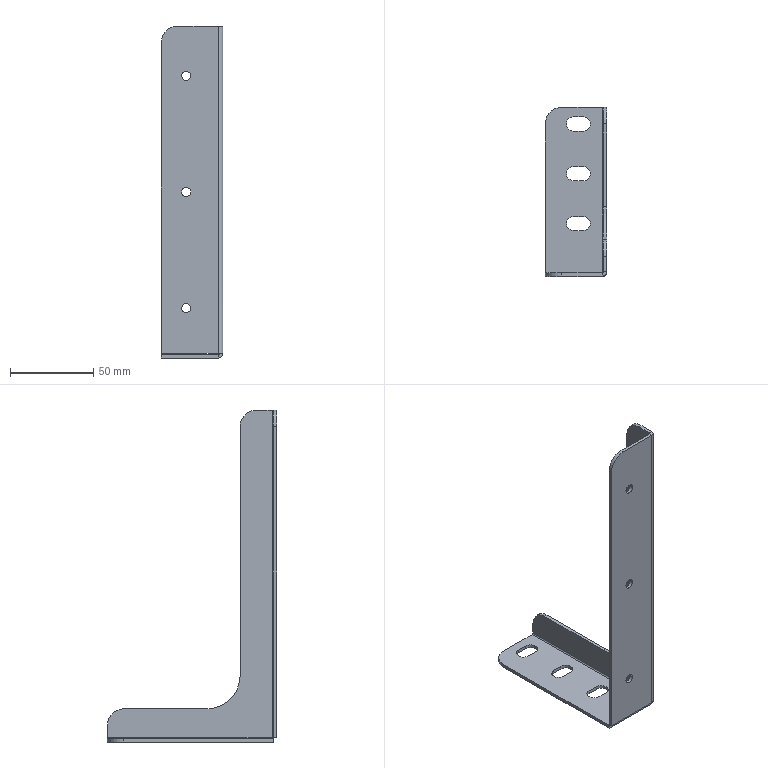Part | STEP file | 09-35 right support plate (Default) | 1 solid | 51 faces | box 37 x 102 x 200 mm | volume 31565 mm3 | plane 27 | cylinder 24 | commonest cylinder face diameters 8.5 x9 5.5 x6 20 x4 1.473 x2 5.473 x2 40 x1
STEP:
#1=CARTESIAN_POINT('',(9.75,-20.,-2.));
#2=VERTEX_POINT('',#1);
#3=CARTESIAN_POINT('',(5.5,-15.75,-2.));
#4=VERTEX_POINT('',#3);
#5=CARTESIAN_POINT('',(5.5,-20.,-2.));
#6=DIRECTION('',(0.,0.,1.));
#7=DIRECTION('',(1.,0.,0.));
#8=AXIS2_PLACEMENT_3D('',#5,#6,#7);
#9=CIRCLE('',#8,4.25);
#10=EDGE_CURVE('',#2,#4,#9,.T.);
#11=ORIENTED_EDGE('',*,*,#10,.F.);
#12=CARTESIAN_POINT('',(9.75,-20.,0.));
#13=VERTEX_POINT('',#12);
#14=CARTESIAN_POINT('',(9.75,-20.,-10.));
#15=DIRECTION('',(0.,0.,1.));
#16=VECTOR('',#15,1000.);
#17=LINE('',#14,#16);
#18=EDGE_CURVE('',#2,#13,#17,.T.);
#19=ORIENTED_EDGE('',*,*,#18,.T.);
#20=CARTESIAN_POINT('',(5.5,-15.75,0.));
#21=VERTEX_POINT('',#20);
#22=CARTESIAN_POINT('',(5.5,-20.,0.));
#23=DIRECTION('',(0.,0.,1.));
#24=DIRECTION('',(1.,0.,0.));
#25=AXIS2_PLACEMENT_3D('',#22,#23,#24);
#26=CIRCLE('',#25,4.25);
#27=EDGE_CURVE('',#13,#21,#26,.T.);
#28=ORIENTED_EDGE('',*,*,#27,.T.);
#29=CARTESIAN_POINT('',(5.5,-15.75,-10.));
#30=DIRECTION('',(0.,0.,1.));
#31=VECTOR('',#30,1000.);
#32=LINE('',#29,#31);
#33=EDGE_CURVE('',#4,#21,#32,.T.);
#34=ORIENTED_EDGE('',*,*,#33,.F.);
#35=EDGE_LOOP('',(#11,#19,#28,#34));
#36=FACE_OUTER_BOUND('',#35,.T.);
#37=CARTESIAN_POINT('',(5.5,-20.,-10.));
#38=DIRECTION('',(0.,0.,1.));
#39=DIRECTION('',(1.,0.,0.));
#40=AXIS2_PLACEMENT_3D('',#37,#38,#39);
#41=CYLINDRICAL_SURFACE('',#40,4.25);
#42=ADVANCED_FACE('',(#36),#41,.F.);
#43=CARTESIAN_POINT('',(9.75,10.,-2.));
#44=VERTEX_POINT('',#43);
#45=CARTESIAN_POINT('',(5.5,14.25,-2.));
#46=VERTEX_POINT('',#45);
#47=CARTESIAN_POINT('',(5.5,10.,-2.));
#48=DIRECTION('',(0.,0.,1.));
#49=DIRECTION('',(1.,0.,0.));
#50=AXIS2_PLACEMENT_3D('',#47,#48,#49);
#51=CIRCLE('',#50,4.25);
#52=EDGE_CURVE('',#44,#46,#51,.T.);
#53=ORIENTED_EDGE('',*,*,#52,.F.);
#54=CARTESIAN_POINT('',(9.75,10.,0.));
#55=VERTEX_POINT('',#54);
#56=CARTESIAN_POINT('',(9.75,10.,-10.));
#57=DIRECTION('',(0.,0.,1.));
#58=VECTOR('',#57,1000.);
#59=LINE('',#56,#58);
#60=EDGE_CURVE('',#44,#55,#59,.T.);
#61=ORIENTED_EDGE('',*,*,#60,.T.);
#62=CARTESIAN_POINT('',(5.5,14.25,0.));
#63=VERTEX_POINT('',#62);
#64=CARTESIAN_POINT('',(5.5,10.,0.));
#65=DIRECTION('',(0.,0.,1.));
#66=DIRECTION('',(1.,0.,0.));
#67=AXIS2_PLACEMENT_3D('',#64,#65,#66);
#68=CIRCLE('',#67,4.25);
#69=EDGE_CURVE('',#55,#63,#68,.T.);
#70=ORIENTED_EDGE('',*,*,#69,.T.);
#71=CARTESIAN_POINT('',(5.5,14.25,-10.));
#72=DIRECTION('',(0.,0.,1.));
#73=VECTOR('',#72,1000.);
#74=LINE('',#71,#73);
#75=EDGE_CURVE('',#46,#63,#74,.T.);
#76=ORIENTED_EDGE('',*,*,#75,.F.);
#77=EDGE_LOOP('',(#53,#61,#70,#76));
#78=FACE_OUTER_BOUND('',#77,.T.);
#79=CARTESIAN_POINT('',(5.5,10.,-10.));
#80=DIRECTION('',(0.,0.,1.));
#81=DIRECTION('',(1.,0.,0.));
#82=AXIS2_PLACEMENT_3D('',#79,#80,#81);
#83=CYLINDRICAL_SURFACE('',#82,4.25);
#84=ADVANCED_FACE('',(#78),#83,.F.);
#85=CARTESIAN_POINT('',(9.75,40.,-2.));
#86=VERTEX_POINT('',#85);
#87=CARTESIAN_POINT('',(5.5,44.25,-2.));
#88=VERTEX_POINT('',#87);
#89=CARTESIAN_POINT('',(5.5,40.,-2.));
#90=DIRECTION('',(0.,0.,1.));
#91=DIRECTION('',(1.,0.,0.));
#92=AXIS2_PLACEMENT_3D('',#89,#90,#91);
#93=CIRCLE('',#92,4.25);
#94=EDGE_CURVE('',#86,#88,#93,.T.);
#95=ORIENTED_EDGE('',*,*,#94,.F.);
#96=CARTESIAN_POINT('',(9.75,40.,0.));
#97=VERTEX_POINT('',#96);
#98=CARTESIAN_POINT('',(9.75,40.,-10.));
#99=DIRECTION('',(0.,0.,1.));
#100=VECTOR('',#99,1000.);
#101=LINE('',#98,#100);
#102=EDGE_CURVE('',#86,#97,#101,.T.);
#103=ORIENTED_EDGE('',*,*,#102,.T.);
#104=CARTESIAN_POINT('',(5.5,44.25,0.));
#105=VERTEX_POINT('',#104);
#106=CARTESIAN_POINT('',(5.5,40.,0.));
#107=DIRECTION('',(0.,0.,1.));
#108=DIRECTION('',(1.,0.,0.));
#109=AXIS2_PLACEMENT_3D('',#106,#107,#108);
#110=CIRCLE('',#109,4.25);
#111=EDGE_CURVE('',#97,#105,#110,.T.);
#112=ORIENTED_EDGE('',*,*,#111,.T.);
#113=CARTESIAN_POINT('',(5.5,44.25,-10.));
#114=DIRECTION('',(0.,0.,1.));
#115=VECTOR('',#114,1000.);
#116=LINE('',#113,#115);
#117=EDGE_CURVE('',#88,#105,#116,.T.);
#118=ORIENTED_EDGE('',*,*,#117,.F.);
#119=EDGE_LOOP('',(#95,#103,#112,#118));
#120=FACE_OUTER_BOUND('',#119,.T.);
#121=CARTESIAN_POINT('',(5.5,40.,-10.));
#122=DIRECTION('',(0.,0.,1.));
#123=DIRECTION('',(1.,0.,0.));
#124=AXIS2_PLACEMENT_3D('',#121,#122,#123);
#125=CYLINDRICAL_SURFACE('',#124,4.25);
#126=ADVANCED_FACE('',(#120),#125,.F.);
#127=CARTESIAN_POINT('',(-5.25,-50.,28.));
#128=VERTEX_POINT('',#127);
#129=CARTESIAN_POINT('',(0.25,-50.,28.));
#130=VERTEX_POINT('',#129);
#131=CARTESIAN_POINT('',(-2.5,-50.,28.));
#132=DIRECTION('',(0.,-1.,0.));
#133=DIRECTION('',(1.,0.,0.));
#134=AXIS2_PLACEMENT_3D('',#131,#132,#133);
#135=CIRCLE('',#134,2.75);
#136=EDGE_CURVE('',#128,#130,#135,.T.);
#137=ORIENTED_EDGE('',*,*,#136,.F.);
#138=CARTESIAN_POINT('',(-5.25,-52.,28.));
#139=VERTEX_POINT('',#138);
#140=CARTESIAN_POINT('',(-5.25,-42.,28.));
#141=DIRECTION('',(0.,-1.,0.));
#142=VECTOR('',#141,1000.);
#143=LINE('',#140,#142);
#144=EDGE_CURVE('',#128,#139,#143,.T.);
#145=ORIENTED_EDGE('',*,*,#144,.T.);
#146=CARTESIAN_POINT('',(0.25,-52.,28.));
#147=VERTEX_POINT('',#146);
#148=CARTESIAN_POINT('',(-2.5,-52.,28.));
#149=DIRECTION('',(0.,-1.,0.));
#150=DIRECTION('',(1.,0.,0.));
#151=AXIS2_PLACEMENT_3D('',#148,#149,#150);
#152=CIRCLE('',#151,2.75);
#153=EDGE_CURVE('',#139,#147,#152,.T.);
#154=ORIENTED_EDGE('',*,*,#153,.T.);
#155=CARTESIAN_POINT('',(0.25,-42.,28.));
#156=DIRECTION('',(0.,-1.,0.));
#157=VECTOR('',#156,1000.);
#158=LINE('',#155,#157);
#159=EDGE_CURVE('',#130,#147,#158,.T.);
#160=ORIENTED_EDGE('',*,*,#159,.F.);
#161=EDGE_LOOP('',(#137,#145,#154,#160));
#162=FACE_OUTER_BOUND('',#161,.T.);
#163=CARTESIAN_POINT('',(-2.5,-42.,28.));
#164=DIRECTION('',(0.,-1.,0.));
#165=DIRECTION('',(1.,0.,0.));
#166=AXIS2_PLACEMENT_3D('',#163,#164,#165);
#167=CYLINDRICAL_SURFACE('',#166,2.75);
#168=ADVANCED_FACE('',(#162),#167,.F.);
#169=CARTESIAN_POINT('',(-5.25,-50.,98.));
#170=VERTEX_POINT('',#169);
#171=CARTESIAN_POINT('',(0.25,-50.,98.));
#172=VERTEX_POINT('',#171);
#173=CARTESIAN_POINT('',(-2.5,-50.,98.));
#174=DIRECTION('',(0.,-1.,0.));
#175=DIRECTION('',(1.,0.,0.));
#176=AXIS2_PLACEMENT_3D('',#173,#174,#175);
#177=CIRCLE('',#176,2.75);
#178=EDGE_CURVE('',#170,#172,#177,.T.);
#179=ORIENTED_EDGE('',*,*,#178,.F.);
#180=CARTESIAN_POINT('',(-5.25,-52.,98.));
#181=VERTEX_POINT('',#180);
#182=CARTESIAN_POINT('',(-5.25,-42.,98.));
#183=DIRECTION('',(0.,-1.,0.));
#184=VECTOR('',#183,1000.);
#185=LINE('',#182,#184);
#186=EDGE_CURVE('',#170,#181,#185,.T.);
#187=ORIENTED_EDGE('',*,*,#186,.T.);
#188=CARTESIAN_POINT('',(0.25,-52.,98.));
#189=VERTEX_POINT('',#188);
#190=CARTESIAN_POINT('',(-2.5,-52.,98.));
#191=DIRECTION('',(0.,-1.,0.));
#192=DIRECTION('',(1.,0.,0.));
#193=AXIS2_PLACEMENT_3D('',#190,#191,#192);
#194=CIRCLE('',#193,2.75);
#195=EDGE_CURVE('',#181,#189,#194,.T.);
#196=ORIENTED_EDGE('',*,*,#195,.T.);
#197=CARTESIAN_POINT('',(0.25,-42.,98.));
#198=DIRECTION('',(0.,-1.,0.));
#199=VECTOR('',#198,1000.);
#200=LINE('',#197,#199);
#201=EDGE_CURVE('',#172,#189,#200,.T.);
#202=ORIENTED_EDGE('',*,*,#201,.F.);
#203=EDGE_LOOP('',(#179,#187,#196,#202));
#204=FACE_OUTER_BOUND('',#203,.T.);
#205=CARTESIAN_POINT('',(-2.5,-42.,98.));
#206=DIRECTION('',(0.,-1.,0.));
#207=DIRECTION('',(1.,0.,0.));
#208=AXIS2_PLACEMENT_3D('',#205,#206,#207);
#209=CYLINDRICAL_SURFACE('',#208,2.75);
#210=ADVANCED_FACE('',(#204),#209,.F.);
#211=CARTESIAN_POINT('',(-5.25,-50.,168.));
#212=VERTEX_POINT('',#211);
#213=CARTESIAN_POINT('',(0.25,-50.,168.));
#214=VERTEX_POINT('',#213);
#215=CARTESIAN_POINT('',(-2.5,-50.,168.));
#216=DIRECTION('',(0.,-1.,0.));
#217=DIRECTION('',(1.,0.,0.));
#218=AXIS2_PLACEMENT_3D('',#215,#216,#217);
#219=CIRCLE('',#218,2.75);
#220=EDGE_CURVE('',#212,#214,#219,.T.);
#221=ORIENTED_EDGE('',*,*,#220,.F.);
#222=CARTESIAN_POINT('',(-5.25,-52.,168.));
#223=VERTEX_POINT('',#222);
#224=CARTESIAN_POINT('',(-5.25,-42.,168.));
#225=DIRECTION('',(0.,-1.,0.));
#226=VECTOR('',#225,1000.);
#227=LINE('',#224,#226);
#228=EDGE_CURVE('',#212,#223,#227,.T.);
#229=ORIENTED_EDGE('',*,*,#228,.T.);
#230=CARTESIAN_POINT('',(0.25,-52.,168.));
#231=VERTEX_POINT('',#230);
#232=CARTESIAN_POINT('',(-2.5,-52.,168.));
#233=DIRECTION('',(0.,-1.,0.));
#234=DIRECTION('',(1.,0.,0.));
#235=AXIS2_PLACEMENT_3D('',#232,#233,#234);
#236=CIRCLE('',#235,2.75);
#237=EDGE_CURVE('',#223,#231,#236,.T.);
#238=ORIENTED_EDGE('',*,*,#237,.T.);
#239=CARTESIAN_POINT('',(0.25,-42.,168.));
#240=DIRECTION('',(0.,-1.,0.));
#241=VECTOR('',#240,1000.);
#242=LINE('',#239,#241);
#243=EDGE_CURVE('',#214,#231,#242,.T.);
#244=ORIENTED_EDGE('',*,*,#243,.F.);
#245=EDGE_LOOP('',(#221,#229,#238,#244));
#246=FACE_OUTER_BOUND('',#245,.T.);
#247=CARTESIAN_POINT('',(-2.5,-42.,168.));
#248=DIRECTION('',(0.,-1.,0.));
#249=DIRECTION('',(1.,0.,0.));
#250=AXIS2_PLACEMENT_3D('',#247,#248,#249);
#251=CYLINDRICAL_SURFACE('',#250,2.75);
#252=ADVANCED_FACE('',(#246),#251,.F.);
#253=CARTESIAN_POINT('',(19.5,-50.,0.7366));
#254=VERTEX_POINT('',#253);
#255=CARTESIAN_POINT('',(19.5,-49.263,0.7366));
#256=VERTEX_POINT('',#255);
#257=CARTESIAN_POINT('',(19.5,50.,0.7366));
#258=DIRECTION('',(0.,1.,0.));
#259=VECTOR('',#258,1000.);
#260=LINE('',#257,#259);
#261=EDGE_CURVE('',#254,#256,#260,.T.);
#262=ORIENTED_EDGE('',*,*,#261,.T.);
#263=CARTESIAN_POINT('',(19.399,-50.,0.7366));
#264=VERTEX_POINT('',#263);
#265=CARTESIAN_POINT('',(16.763,-49.263,0.7366));
#266=DIRECTION('',(0.,0.,-1.));
#267=DIRECTION('',(1.,0.,0.));
#268=AXIS2_PLACEMENT_3D('',#265,#266,#267);
#269=CIRCLE('',#268,2.737);
#270=EDGE_CURVE('',#256,#264,#269,.T.);
#271=ORIENTED_EDGE('',*,*,#270,.T.);
#272=CARTESIAN_POINT('',(17.5,-50.,0.7366));
#273=DIRECTION('',(1.,0.,0.));
#274=VECTOR('',#273,1000.);
#275=LINE('',#272,#274);
#276=EDGE_CURVE('',#264,#254,#275,.T.);
#277=ORIENTED_EDGE('',*,*,#276,.T.);
#278=EDGE_LOOP('',(#262,#271,#277));
#279=FACE_OUTER_BOUND('',#278,.T.);
#280=CARTESIAN_POINT('',(17.5,-49.263,0.7366));
#281=DIRECTION('',(0.,0.,1.));
#282=DIRECTION('',(0.,-1.,0.));
#283=AXIS2_PLACEMENT_3D('',#280,#281,#282);
#284=PLANE('',#283);
#285=ADVANCED_FACE('',(#279),#284,.T.);
#286=CARTESIAN_POINT('',(19.5,-30.,188.));
#287=VERTEX_POINT('',#286);
#288=CARTESIAN_POINT('',(19.5,-30.,38.));
#289=VERTEX_POINT('',#288);
#290=CARTESIAN_POINT('',(19.5,-30.,0.));
#291=DIRECTION('',(0.,0.,-1.));
#292=VECTOR('',#291,1000.);
#293=LINE('',#290,#292);
#294=EDGE_CURVE('',#287,#289,#293,.T.);
#295=ORIENTED_EDGE('',*,*,#294,.F.);
#296=CARTESIAN_POINT('',(19.5,-40.,198.));
#297=VERTEX_POINT('',#296);
#298=CARTESIAN_POINT('',(19.5,-40.,188.));
#299=DIRECTION('',(1.,0.,0.));
#300=DIRECTION('',(0.,0.,-1.));
#301=AXIS2_PLACEMENT_3D('',#298,#299,#300);
#302=CIRCLE('',#301,10.);
#303=EDGE_CURVE('',#287,#297,#302,.T.);
#304=ORIENTED_EDGE('',*,*,#303,.T.);
#305=CARTESIAN_POINT('',(19.5,-49.263,198.));
#306=VERTEX_POINT('',#305);
#307=CARTESIAN_POINT('',(19.5,50.,198.));
#308=DIRECTION('',(0.,1.,0.));
#309=VECTOR('',#308,1000.);
#310=LINE('',#307,#309);
#311=EDGE_CURVE('',#306,#297,#310,.T.);
#312=ORIENTED_EDGE('',*,*,#311,.F.);
#313=CARTESIAN_POINT('',(19.5,-49.263,198.));
#314=DIRECTION('',(0.,0.,-1.));
#315=VECTOR('',#314,1000.);
#316=LINE('',#313,#315);
#317=EDGE_CURVE('',#306,#256,#316,.T.);
#318=ORIENTED_EDGE('',*,*,#317,.T.);
#319=CARTESIAN_POINT('',(19.5,50.,0.7366));
#320=VERTEX_POINT('',#319);
#321=CARTESIAN_POINT('',(19.5,50.,0.7366));
#322=DIRECTION('',(0.,1.,0.));
#323=VECTOR('',#322,1000.);
#324=LINE('',#321,#323);
#325=EDGE_CURVE('',#256,#320,#324,.T.);
#326=ORIENTED_EDGE('',*,*,#325,.T.);
#327=CARTESIAN_POINT('',(19.5,50.,8.));
#328=VERTEX_POINT('',#327);
#329=CARTESIAN_POINT('',(19.5,50.,0.));
#330=DIRECTION('',(0.,0.,-1.));
#331=VECTOR('',#330,1000.);
#332=LINE('',#329,#331);
#333=EDGE_CURVE('',#328,#320,#332,.T.);
#334=ORIENTED_EDGE('',*,*,#333,.F.);
#335=CARTESIAN_POINT('',(19.5,40.,18.));
#336=VERTEX_POINT('',#335);
#337=CARTESIAN_POINT('',(19.5,40.,8.));
#338=DIRECTION('',(1.,0.,0.));
#339=DIRECTION('',(0.,0.,-1.));
#340=AXIS2_PLACEMENT_3D('',#337,#338,#339);
#341=CIRCLE('',#340,10.);
#342=EDGE_CURVE('',#328,#336,#341,.T.);
#343=ORIENTED_EDGE('',*,*,#342,.T.);
#344=CARTESIAN_POINT('',(19.5,-10.,18.));
#345=VERTEX_POINT('',#344);
#346=CARTESIAN_POINT('',(19.5,50.,18.));
#347=DIRECTION('',(0.,1.,0.));
#348=VECTOR('',#347,1000.);
#349=LINE('',#346,#348);
#350=EDGE_CURVE('',#345,#336,#349,.T.);
#351=ORIENTED_EDGE('',*,*,#350,.F.);
#352=CARTESIAN_POINT('',(19.5,-10.,38.));
#353=DIRECTION('',(1.,0.,0.));
#354=DIRECTION('',(0.,0.,-1.));
#355=AXIS2_PLACEMENT_3D('',#352,#353,#354);
#356=CIRCLE('',#355,20.);
#357=EDGE_CURVE('',#289,#345,#356,.T.);
#358=ORIENTED_EDGE('',*,*,#357,.F.);
#359=EDGE_LOOP('',(#295,#304,#312,#318,#326,#334,#343,#351,#358));
#360=FACE_OUTER_BOUND('',#359,.T.);
#361=CARTESIAN_POINT('',(19.5,50.,0.));
#362=DIRECTION('',(1.,0.,0.));
#363=DIRECTION('',(0.,0.,-1.));
#364=AXIS2_PLACEMENT_3D('',#361,#362,#363);
#365=PLANE('',#364);
#366=ADVANCED_FACE('',(#360),#365,.T.);
#367=CARTESIAN_POINT('',(17.5,-49.263,198.));
#368=VERTEX_POINT('',#367);
#369=CARTESIAN_POINT('',(17.5,-40.,198.));
#370=VERTEX_POINT('',#369);
#371=CARTESIAN_POINT('',(17.5,50.,198.));
#372=DIRECTION('',(0.,1.,0.));
#373=VECTOR('',#372,1000.);
#374=LINE('',#371,#373);
#375=EDGE_CURVE('',#368,#370,#374,.T.);
#376=ORIENTED_EDGE('',*,*,#375,.T.);
#377=CARTESIAN_POINT('',(17.5,-30.,188.));
#378=VERTEX_POINT('',#377);
#379=CARTESIAN_POINT('',(17.5,-40.,188.));
#380=DIRECTION('',(-1.,0.,0.));
#381=DIRECTION('',(0.,0.,-1.));
#382=AXIS2_PLACEMENT_3D('',#379,#380,#381);
#383=CIRCLE('',#382,10.);
#384=EDGE_CURVE('',#370,#378,#383,.T.);
#385=ORIENTED_EDGE('',*,*,#384,.T.);
#386=CARTESIAN_POINT('',(17.5,-30.,38.));
#387=VERTEX_POINT('',#386);
#388=CARTESIAN_POINT('',(17.5,-30.,198.));
#389=DIRECTION('',(0.,0.,1.));
#390=VECTOR('',#389,1000.);
#391=LINE('',#388,#390);
#392=EDGE_CURVE('',#387,#378,#391,.T.);
#393=ORIENTED_EDGE('',*,*,#392,.F.);
#394=CARTESIAN_POINT('',(17.5,-10.,18.));
#395=VERTEX_POINT('',#394);
#396=CARTESIAN_POINT('',(17.5,-10.,38.));
#397=DIRECTION('',(-1.,0.,0.));
#398=DIRECTION('',(0.,0.,1.));
#399=AXIS2_PLACEMENT_3D('',#396,#397,#398);
#400=CIRCLE('',#399,20.);
#401=EDGE_CURVE('',#395,#387,#400,.T.);
#402=ORIENTED_EDGE('',*,*,#401,.F.);
#403=CARTESIAN_POINT('',(17.5,40.,18.));
#404=VERTEX_POINT('',#403);
#405=CARTESIAN_POINT('',(17.5,50.,18.));
#406=DIRECTION('',(0.,-1.,0.));
#407=VECTOR('',#406,1000.);
#408=LINE('',#405,#407);
#409=EDGE_CURVE('',#404,#395,#408,.T.);
#410=ORIENTED_EDGE('',*,*,#409,.F.);
#411=CARTESIAN_POINT('',(17.5,50.,8.));
#412=VERTEX_POINT('',#411);
#413=CARTESIAN_POINT('',(17.5,40.,8.));
#414=DIRECTION('',(-1.,0.,0.));
#415=DIRECTION('',(0.,0.,-1.));
#416=AXIS2_PLACEMENT_3D('',#413,#414,#415);
#417=CIRCLE('',#416,10.);
#418=EDGE_CURVE('',#404,#412,#417,.T.);
#419=ORIENTED_EDGE('',*,*,#418,.T.);
#420=CARTESIAN_POINT('',(17.5,50.,0.7366));
#421=VERTEX_POINT('',#420);
#422=CARTESIAN_POINT('',(17.5,50.,0.));
#423=DIRECTION('',(0.,0.,-1.));
#424=VECTOR('',#423,1000.);
#425=LINE('',#422,#424);
#426=EDGE_CURVE('',#412,#421,#425,.T.);
#427=ORIENTED_EDGE('',*,*,#426,.T.);
#428=CARTESIAN_POINT('',(17.5,-49.263,0.7366));
#429=VERTEX_POINT('',#428);
#430=CARTESIAN_POINT('',(17.5,-50.,0.7366));
#431=DIRECTION('',(0.,1.,0.));
#432=VECTOR('',#431,1000.);
#433=LINE('',#430,#432);
#434=EDGE_CURVE('',#429,#421,#433,.T.);
#435=ORIENTED_EDGE('',*,*,#434,.F.);
#436=CARTESIAN_POINT('',(17.5,-49.263,198.));
#437=DIRECTION('',(0.,0.,-1.));
#438=VECTOR('',#437,1000.);
#439=LINE('',#436,#438);
#440=EDGE_CURVE('',#368,#429,#439,.T.);
#441=ORIENTED_EDGE('',*,*,#440,.F.);
#442=EDGE_LOOP('',(#376,#385,#393,#402,#410,#419,#427,#435,#441));
#443=FACE_OUTER_BOUND('',#442,.T.);
#444=CARTESIAN_POINT('',(17.5,50.,0.));
#445=DIRECTION('',(1.,0.,0.));
#446=DIRECTION('',(0.,0.,-1.));
#447=AXIS2_PLACEMENT_3D('',#444,#445,#446);
#448=PLANE('',#447);
#449=ADVANCED_FACE('',(#443),#448,.F.);
#450=ORIENTED_EDGE('',*,*,#311,.T.);
#451=CARTESIAN_POINT('',(17.5,-40.,198.));
#452=DIRECTION('',(-1.,0.,0.));
#453=VECTOR('',#452,1000.);
#454=LINE('',#451,#453);
#455=EDGE_CURVE('',#297,#370,#454,.T.);
#456=ORIENTED_EDGE('',*,*,#455,.T.);
#457=ORIENTED_EDGE('',*,*,#375,.F.);
#458=CARTESIAN_POINT('',(17.5,-49.263,198.));
#459=DIRECTION('',(1.,0.,0.));
#460=VECTOR('',#459,1000.);
#461=LINE('',#458,#460);
#462=EDGE_CURVE('',#368,#306,#461,.T.);
#463=ORIENTED_EDGE('',*,*,#462,.T.);
#464=EDGE_LOOP('',(#450,#456,#457,#463));
#465=FACE_OUTER_BOUND('',#464,.T.);
#466=CARTESIAN_POINT('',(19.5,50.,198.));
#467=DIRECTION('',(0.,0.,1.));
#468=DIRECTION('',(1.,0.,0.));
#469=AXIS2_PLACEMENT_3D('',#466,#467,#468);
#470=PLANE('',#469);
#471=ADVANCED_FACE('',(#465),#470,.T.);
#472=CARTESIAN_POINT('',(16.763,50.,-2.));
#473=VERTEX_POINT('',#472);
#474=CARTESIAN_POINT('',(-7.5,50.,-2.));
#475=VERTEX_POINT('',#474);
#476=CARTESIAN_POINT('',(-17.5,50.,-2.));
#477=DIRECTION('',(-1.,0.,0.));
#478=VECTOR('',#477,1000.);
#479=LINE('',#476,#478);
#480=EDGE_CURVE('',#473,#475,#479,.T.);
#481=ORIENTED_EDGE('',*,*,#480,.T.);
#482=CARTESIAN_POINT('',(-7.5,50.,0.));
#483=VERTEX_POINT('',#482);
#484=CARTESIAN_POINT('',(-7.5,50.,-2.));
#485=DIRECTION('',(0.,0.,1.));
#486=VECTOR('',#485,1000.);
#487=LINE('',#484,#486);
#488=EDGE_CURVE('',#475,#483,#487,.T.);
#489=ORIENTED_EDGE('',*,*,#488,.T.);
#490=CARTESIAN_POINT('',(16.763,50.,0.));
#491=VERTEX_POINT('',#490);
#492=CARTESIAN_POINT('',(-17.5,50.,0.));
#493=DIRECTION('',(-1.,0.,0.));
#494=VECTOR('',#493,1000.);
#495=LINE('',#492,#494);
#496=EDGE_CURVE('',#491,#483,#495,.T.);
#497=ORIENTED_EDGE('',*,*,#496,.F.);
#498=CARTESIAN_POINT('',(16.763,50.,0.));
#499=DIRECTION('',(0.,0.,-1.));
#500=VECTOR('',#499,1000.);
#501=LINE('',#498,#500);
#502=EDGE_CURVE('',#491,#473,#501,.T.);
#503=ORIENTED_EDGE('',*,*,#502,.T.);
#504=EDGE_LOOP('',(#481,#489,#497,#503));
#505=FACE_OUTER_BOUND('',#504,.T.);
#506=CARTESIAN_POINT('',(-17.5,50.,-2.));
#507=DIRECTION('',(0.,1.,0.));
#508=DIRECTION('',(0.,0.,1.));
#509=AXIS2_PLACEMENT_3D('',#506,#507,#508);
#510=PLANE('',#509);
#511=ADVANCED_FACE('',(#505),#510,.T.);
#512=CARTESIAN_POINT('',(-0.5,-15.75,-2.));
#513=VERTEX_POINT('',#512);
#514=CARTESIAN_POINT('',(17.5,-15.75,-2.));
#515=DIRECTION('',(-1.,0.,0.));
#516=VECTOR('',#515,1000.);
#517=LINE('',#514,#516);
#518=EDGE_CURVE('',#4,#513,#517,.T.);
#519=ORIENTED_EDGE('',*,*,#518,.T.);
#520=CARTESIAN_POINT('',(-0.5,-24.25,-2.));
#521=VERTEX_POINT('',#520);
#522=CARTESIAN_POINT('',(-0.5,-20.,-2.));
#523=DIRECTION('',(0.,0.,1.));
#524=DIRECTION('',(1.,0.,0.));
#525=AXIS2_PLACEMENT_3D('',#522,#523,#524);
#526=CIRCLE('',#525,4.25);
#527=EDGE_CURVE('',#513,#521,#526,.T.);
#528=ORIENTED_EDGE('',*,*,#527,.T.);
#529=CARTESIAN_POINT('',(5.5,-24.25,-2.));
#530=VERTEX_POINT('',#529);
#531=CARTESIAN_POINT('',(17.5,-24.25,-2.));
#532=DIRECTION('',(1.,0.,0.));
#533=VECTOR('',#532,1000.);
#534=LINE('',#531,#533);
#535=EDGE_CURVE('',#521,#530,#534,.T.);
#536=ORIENTED_EDGE('',*,*,#535,.T.);
#537=CARTESIAN_POINT('',(5.5,-20.,-2.));
#538=DIRECTION('',(0.,0.,1.));
#539=DIRECTION('',(1.,0.,0.));
#540=AXIS2_PLACEMENT_3D('',#537,#538,#539);
#541=CIRCLE('',#540,4.25);
#542=EDGE_CURVE('',#530,#2,#541,.T.);
#543=ORIENTED_EDGE('',*,*,#542,.T.);
#544=ORIENTED_EDGE('',*,*,#10,.T.);
#545=EDGE_LOOP('',(#519,#528,#536,#543,#544));
#546=FACE_BOUND('',#545,.T.);
#547=CARTESIAN_POINT('',(-0.5,14.25,-2.));
#548=VERTEX_POINT('',#547);
#549=CARTESIAN_POINT('',(17.5,14.25,-2.));
#550=DIRECTION('',(-1.,0.,0.));
#551=VECTOR('',#550,1000.);
#552=LINE('',#549,#551);
#553=EDGE_CURVE('',#46,#548,#552,.T.);
#554=ORIENTED_EDGE('',*,*,#553,.T.);
#555=CARTESIAN_POINT('',(-0.5,5.75,-2.));
#556=VERTEX_POINT('',#555);
#557=CARTESIAN_POINT('',(-0.5,10.,-2.));
#558=DIRECTION('',(0.,0.,1.));
#559=DIRECTION('',(1.,0.,0.));
#560=AXIS2_PLACEMENT_3D('',#557,#558,#559);
#561=CIRCLE('',#560,4.25);
#562=EDGE_CURVE('',#548,#556,#561,.T.);
#563=ORIENTED_EDGE('',*,*,#562,.T.);
#564=CARTESIAN_POINT('',(5.5,5.75,-2.));
#565=VERTEX_POINT('',#564);
#566=CARTESIAN_POINT('',(17.5,5.75,-2.));
#567=DIRECTION('',(1.,0.,0.));
#568=VECTOR('',#567,1000.);
#569=LINE('',#566,#568);
#570=EDGE_CURVE('',#556,#565,#569,.T.);
#571=ORIENTED_EDGE('',*,*,#570,.T.);
#572=CARTESIAN_POINT('',(5.5,10.,-2.));
#573=DIRECTION('',(0.,0.,1.));
#574=DIRECTION('',(1.,0.,0.));
#575=AXIS2_PLACEMENT_3D('',#572,#573,#574);
#576=CIRCLE('',#575,4.25);
#577=EDGE_CURVE('',#565,#44,#576,.T.);
#578=ORIENTED_EDGE('',*,*,#577,.T.);
#579=ORIENTED_EDGE('',*,*,#52,.T.);
#580=EDGE_LOOP('',(#554,#563,#571,#578,#579));
#581=FACE_BOUND('',#580,.T.);
#582=CARTESIAN_POINT('',(-0.5,44.25,-2.));
#583=VERTEX_POINT('',#582);
#584=CARTESIAN_POINT('',(17.5,44.25,-2.));
#585=DIRECTION('',(-1.,0.,0.));
#586=VECTOR('',#585,1000.);
#587=LINE('',#584,#586);
#588=EDGE_CURVE('',#88,#583,#587,.T.);
#589=ORIENTED_EDGE('',*,*,#588,.T.);
#590=CARTESIAN_POINT('',(-0.5,35.75,-2.));
#591=VERTEX_POINT('',#590);
#592=CARTESIAN_POINT('',(-0.5,40.,-2.));
#593=DIRECTION('',(0.,0.,1.));
#594=DIRECTION('',(1.,0.,0.));
#595=AXIS2_PLACEMENT_3D('',#592,#593,#594);
#596=CIRCLE('',#595,4.25);
#597=EDGE_CURVE('',#583,#591,#596,.T.);
#598=ORIENTED_EDGE('',*,*,#597,.T.);
#599=CARTESIAN_POINT('',(5.5,35.75,-2.));
#600=VERTEX_POINT('',#599);
#601=CARTESIAN_POINT('',(17.5,35.75,-2.));
#602=DIRECTION('',(1.,0.,0.));
#603=VECTOR('',#602,1000.);
#604=LINE('',#601,#603);
#605=EDGE_CURVE('',#591,#600,#604,.T.);
#606=ORIENTED_EDGE('',*,*,#605,.T.);
#607=CARTESIAN_POINT('',(5.5,40.,-2.));
#608=DIRECTION('',(0.,0.,1.));
#609=DIRECTION('',(1.,0.,0.));
#610=AXIS2_PLACEMENT_3D('',#607,#608,#609);
#611=CIRCLE('',#610,4.25);
#612=EDGE_CURVE('',#600,#86,#611,.T.);
#613=ORIENTED_EDGE('',*,*,#612,.T.);
#614=ORIENTED_EDGE('',*,*,#94,.T.);
#615=EDGE_LOOP('',(#589,#598,#606,#613,#614));
#616=FACE_BOUND('',#615,.T.);
#617=CARTESIAN_POINT('',(-17.5,40.,-2.));
#618=VERTEX_POINT('',#617);
#619=CARTESIAN_POINT('',(-17.5,-50.,-2.));
#620=VERTEX_POINT('',#619);
#621=CARTESIAN_POINT('',(-17.5,50.,-2.));
#622=DIRECTION('',(0.,-1.,0.));
#623=VECTOR('',#622,1000.);
#624=LINE('',#621,#623);
#625=EDGE_CURVE('',#618,#620,#624,.T.);
#626=ORIENTED_EDGE('',*,*,#625,.F.);
#627=CARTESIAN_POINT('',(-7.5,40.,-2.));
#628=DIRECTION('',(0.,0.,-1.));
#629=DIRECTION('',(1.,0.,0.));
#630=AXIS2_PLACEMENT_3D('',#627,#628,#629);
#631=CIRCLE('',#630,10.);
#632=EDGE_CURVE('',#618,#475,#631,.T.);
#633=ORIENTED_EDGE('',*,*,#632,.T.);
#634=ORIENTED_EDGE('',*,*,#480,.F.);
#635=CARTESIAN_POINT('',(16.763,-50.,-2.));
#636=VERTEX_POINT('',#635);
#637=CARTESIAN_POINT('',(16.763,50.,-2.));
#638=DIRECTION('',(0.,-1.,0.));
#639=VECTOR('',#638,1000.);
#640=LINE('',#637,#639);
#641=EDGE_CURVE('',#473,#636,#640,.T.);
#642=ORIENTED_EDGE('',*,*,#641,.T.);
#643=CARTESIAN_POINT('',(-17.5,-50.,-2.));
#644=DIRECTION('',(1.,0.,0.));
#645=VECTOR('',#644,1000.);
#646=LINE('',#643,#645);
#647=EDGE_CURVE('',#620,#636,#646,.T.);
#648=ORIENTED_EDGE('',*,*,#647,.F.);
#649=EDGE_LOOP('',(#626,#633,#634,#642,#648));
#650=FACE_OUTER_BOUND('',#649,.T.);
#651=CARTESIAN_POINT('',(17.5,-50.,-2.));
#652=DIRECTION('',(0.,0.,1.));
#653=DIRECTION('',(1.,0.,0.));
#654=AXIS2_PLACEMENT_3D('',#651,#652,#653);
#655=PLANE('',#654);
#656=ADVANCED_FACE('',(#546,#581,#616,#650),#655,.F.);
#657=CARTESIAN_POINT('',(-0.5,-15.75,0.));
#658=VERTEX_POINT('',#657);
#659=CARTESIAN_POINT('',(-0.5,-24.25,0.));
#660=VERTEX_POINT('',#659);
#661=CARTESIAN_POINT('',(-0.5,-20.,0.));
#662=DIRECTION('',(0.,0.,1.));
#663=DIRECTION('',(1.,0.,0.));
#664=AXIS2_PLACEMENT_3D('',#661,#662,#663);
#665=CIRCLE('',#664,4.25);
#666=EDGE_CURVE('',#658,#660,#665,.T.);
#667=ORIENTED_EDGE('',*,*,#666,.F.);
#668=CARTESIAN_POINT('',(-0.5,-15.75,0.));
#669=DIRECTION('',(-1.,0.,0.));
#670=VECTOR('',#669,1000.);
#671=LINE('',#668,#670);
#672=EDGE_CURVE('',#21,#658,#671,.T.);
#673=ORIENTED_EDGE('',*,*,#672,.F.);
#674=ORIENTED_EDGE('',*,*,#27,.F.);
#675=CARTESIAN_POINT('',(5.5,-24.25,0.));
#676=VERTEX_POINT('',#675);
#677=CARTESIAN_POINT('',(5.5,-20.,0.));
#678=DIRECTION('',(0.,0.,1.));
#679=DIRECTION('',(1.,0.,0.));
#680=AXIS2_PLACEMENT_3D('',#677,#678,#679);
#681=CIRCLE('',#680,4.25);
#682=EDGE_CURVE('',#676,#13,#681,.T.);
#683=ORIENTED_EDGE('',*,*,#682,.F.);
#684=CARTESIAN_POINT('',(-0.5,-24.25,0.));
#685=DIRECTION('',(1.,0.,0.));
#686=VECTOR('',#685,1000.);
#687=LINE('',#684,#686);
#688=EDGE_CURVE('',#660,#676,#687,.T.);
#689=ORIENTED_EDGE('',*,*,#688,.F.);
#690=EDGE_LOOP('',(#667,#673,#674,#683,#689));
#691=FACE_BOUND('',#690,.T.);
#692=CARTESIAN_POINT('',(-0.5,14.25,0.));
#693=VERTEX_POINT('',#692);
#694=CARTESIAN_POINT('',(-0.5,5.75,0.));
#695=VERTEX_POINT('',#694);
#696=CARTESIAN_POINT('',(-0.5,10.,0.));
#697=DIRECTION('',(0.,0.,1.));
#698=DIRECTION('',(1.,0.,0.));
#699=AXIS2_PLACEMENT_3D('',#696,#697,#698);
#700=CIRCLE('',#699,4.25);
#701=EDGE_CURVE('',#693,#695,#700,.T.);
#702=ORIENTED_EDGE('',*,*,#701,.F.);
#703=CARTESIAN_POINT('',(-0.5,14.25,0.));
#704=DIRECTION('',(-1.,0.,0.));
#705=VECTOR('',#704,1000.);
#706=LINE('',#703,#705);
#707=EDGE_CURVE('',#63,#693,#706,.T.);
#708=ORIENTED_EDGE('',*,*,#707,.F.);
#709=ORIENTED_EDGE('',*,*,#69,.F.);
#710=CARTESIAN_POINT('',(5.5,5.75,0.));
#711=VERTEX_POINT('',#710);
#712=CARTESIAN_POINT('',(5.5,10.,0.));
#713=DIRECTION('',(0.,0.,1.));
#714=DIRECTION('',(1.,0.,0.));
#715=AXIS2_PLACEMENT_3D('',#712,#713,#714);
#716=CIRCLE('',#715,4.25);
#717=EDGE_CURVE('',#711,#55,#716,.T.);
#718=ORIENTED_EDGE('',*,*,#717,.F.);
#719=CARTESIAN_POINT('',(-0.5,5.75,0.));
#720=DIRECTION('',(1.,0.,0.));
#721=VECTOR('',#720,1000.);
#722=LINE('',#719,#721);
#723=EDGE_CURVE('',#695,#711,#722,.T.);
#724=ORIENTED_EDGE('',*,*,#723,.F.);
#725=EDGE_LOOP('',(#702,#708,#709,#718,#724));
#726=FACE_BOUND('',#725,.T.);
#727=CARTESIAN_POINT('',(-0.5,44.25,0.));
#728=VERTEX_POINT('',#727);
#729=CARTESIAN_POINT('',(-0.5,35.75,0.));
#730=VERTEX_POINT('',#729);
#731=CARTESIAN_POINT('',(-0.5,40.,0.));
#732=DIRECTION('',(0.,0.,1.));
#733=DIRECTION('',(1.,0.,0.));
#734=AXIS2_PLACEMENT_3D('',#731,#732,#733);
#735=CIRCLE('',#734,4.25);
#736=EDGE_CURVE('',#728,#730,#735,.T.);
#737=ORIENTED_EDGE('',*,*,#736,.F.);
#738=CARTESIAN_POINT('',(-0.5,44.25,0.));
#739=DIRECTION('',(-1.,0.,0.));
#740=VECTOR('',#739,1000.);
#741=LINE('',#738,#740);
#742=EDGE_CURVE('',#105,#728,#741,.T.);
#743=ORIENTED_EDGE('',*,*,#742,.F.);
#744=ORIENTED_EDGE('',*,*,#111,.F.);
#745=CARTESIAN_POINT('',(5.5,35.75,0.));
#746=VERTEX_POINT('',#745);
#747=CARTESIAN_POINT('',(5.5,40.,0.));
#748=DIRECTION('',(0.,0.,1.));
#749=DIRECTION('',(1.,0.,0.));
#750=AXIS2_PLACEMENT_3D('',#747,#748,#749);
#751=CIRCLE('',#750,4.25);
#752=EDGE_CURVE('',#746,#97,#751,.T.);
#753=ORIENTED_EDGE('',*,*,#752,.F.);
#754=CARTESIAN_POINT('',(-0.5,35.75,0.));
#755=DIRECTION('',(1.,0.,0.));
#756=VECTOR('',#755,1000.);
#757=LINE('',#754,#756);
#758=EDGE_CURVE('',#730,#746,#757,.T.);
#759=ORIENTED_EDGE('',*,*,#758,.F.);
#760=EDGE_LOOP('',(#737,#743,#744,#753,#759));
#761=FACE_BOUND('',#760,.T.);
#762=ORIENTED_EDGE('',*,*,#496,.T.);
#763=CARTESIAN_POINT('',(-17.5,40.,0.));
#764=VERTEX_POINT('',#763);
#765=CARTESIAN_POINT('',(-7.5,40.,0.));
#766=DIRECTION('',(0.,0.,1.));
#767=DIRECTION('',(1.,0.,0.));
#768=AXIS2_PLACEMENT_3D('',#765,#766,#767);
#769=CIRCLE('',#768,10.);
#770=EDGE_CURVE('',#483,#764,#769,.T.);
#771=ORIENTED_EDGE('',*,*,#770,.T.);
#772=CARTESIAN_POINT('',(-17.5,-50.,0.));
#773=VERTEX_POINT('',#772);
#774=CARTESIAN_POINT('',(-17.5,50.,0.));
#775=DIRECTION('',(0.,-1.,0.));
#776=VECTOR('',#775,1000.);
#777=LINE('',#774,#776);
#778=EDGE_CURVE('',#764,#773,#777,.T.);
#779=ORIENTED_EDGE('',*,*,#778,.T.);
#780=CARTESIAN_POINT('',(16.763,-50.,0.));
#781=VERTEX_POINT('',#780);
#782=CARTESIAN_POINT('',(-17.5,-50.,0.));
#783=DIRECTION('',(1.,0.,0.));
#784=VECTOR('',#783,1000.);
#785=LINE('',#782,#784);
#786=EDGE_CURVE('',#773,#781,#785,.T.);
#787=ORIENTED_EDGE('',*,*,#786,.T.);
#788=CARTESIAN_POINT('',(16.763,50.,0.));
#789=DIRECTION('',(0.,-1.,0.));
#790=VECTOR('',#789,1000.);
#791=LINE('',#788,#790);
#792=EDGE_CURVE('',#491,#781,#791,.T.);
#793=ORIENTED_EDGE('',*,*,#792,.F.);
#794=EDGE_LOOP('',(#762,#771,#779,#787,#793));
#795=FACE_OUTER_BOUND('',#794,.T.);
#796=CARTESIAN_POINT('',(17.5,-50.,0.));
#797=DIRECTION('',(0.,0.,1.));
#798=DIRECTION('',(1.,0.,0.));
#799=AXIS2_PLACEMENT_3D('',#796,#797,#798);
#800=PLANE('',#799);
#801=ADVANCED_FACE('',(#691,#726,#761,#795),#800,.T.);
#802=CARTESIAN_POINT('',(16.763,-50.,0.));
#803=DIRECTION('',(0.,0.,-1.));
#804=VECTOR('',#803,1000.);
#805=LINE('',#802,#804);
#806=EDGE_CURVE('',#781,#636,#805,.T.);
#807=ORIENTED_EDGE('',*,*,#806,.F.);
#808=ORIENTED_EDGE('',*,*,#786,.F.);
#809=CARTESIAN_POINT('',(-17.5,-50.,-2.));
#810=DIRECTION('',(0.,0.,1.));
#811=VECTOR('',#810,1000.);
#812=LINE('',#809,#811);
#813=EDGE_CURVE('',#620,#773,#812,.T.);
#814=ORIENTED_EDGE('',*,*,#813,.F.);
#815=ORIENTED_EDGE('',*,*,#647,.T.);
#816=EDGE_LOOP('',(#807,#808,#814,#815));
#817=FACE_OUTER_BOUND('',#816,.T.);
#818=CARTESIAN_POINT('',(-17.5,-50.,-2.));
#819=DIRECTION('',(0.,-1.,0.));
#820=DIRECTION('',(0.,0.,-1.));
#821=AXIS2_PLACEMENT_3D('',#818,#819,#820);
#822=PLANE('',#821);
#823=ADVANCED_FACE('',(#817),#822,.T.);
#824=ORIENTED_EDGE('',*,*,#778,.F.);
#825=CARTESIAN_POINT('',(-17.5,40.,-2.));
#826=DIRECTION('',(0.,0.,-1.));
#827=VECTOR('',#826,1000.);
#828=LINE('',#825,#827);
#829=EDGE_CURVE('',#764,#618,#828,.T.);
#830=ORIENTED_EDGE('',*,*,#829,.T.);
#831=ORIENTED_EDGE('',*,*,#625,.T.);
#832=ORIENTED_EDGE('',*,*,#813,.T.);
#833=EDGE_LOOP('',(#824,#830,#831,#832));
#834=FACE_OUTER_BOUND('',#833,.T.);
#835=CARTESIAN_POINT('',(-17.5,50.,-2.));
#836=DIRECTION('',(-1.,0.,0.));
#837=DIRECTION('',(0.,-1.,0.));
#838=AXIS2_PLACEMENT_3D('',#835,#836,#837);
#839=PLANE('',#838);
#840=ADVANCED_FACE('',(#834),#839,.T.);
#841=CARTESIAN_POINT('',(17.5,-50.,0.7366));
#842=VERTEX_POINT('',#841);
#843=CARTESIAN_POINT('',(17.5,-50.,0.7366));
#844=DIRECTION('',(1.,0.,0.));
#845=VECTOR('',#844,1000.);
#846=LINE('',#843,#845);
#847=EDGE_CURVE('',#842,#264,#846,.T.);
#848=ORIENTED_EDGE('',*,*,#847,.F.);
#849=CARTESIAN_POINT('',(16.763,-50.,0.7366));
#850=DIRECTION('',(0.,-1.,0.));
#851=DIRECTION('',(0.,0.,1.));
#852=AXIS2_PLACEMENT_3D('',#849,#850,#851);
#853=CIRCLE('',#852,0.7366);
#854=EDGE_CURVE('',#781,#842,#853,.T.);
#855=ORIENTED_EDGE('',*,*,#854,.F.);
#856=ORIENTED_EDGE('',*,*,#806,.T.);
#857=CARTESIAN_POINT('',(16.763,-50.,0.7366));
#858=DIRECTION('',(0.,-1.,0.));
#859=DIRECTION('',(0.,0.,1.));
#860=AXIS2_PLACEMENT_3D('',#857,#858,#859);
#861=CIRCLE('',#860,2.737);
#862=EDGE_CURVE('',#636,#254,#861,.T.);
#863=ORIENTED_EDGE('',*,*,#862,.T.);
#864=ORIENTED_EDGE('',*,*,#276,.F.);
#865=EDGE_LOOP('',(#848,#855,#856,#863,#864));
#866=FACE_OUTER_BOUND('',#865,.T.);
#867=CARTESIAN_POINT('',(16.763,-50.,0.7366));
#868=DIRECTION('',(0.,-1.,0.));
#869=DIRECTION('',(0.,0.,-1.));
#870=AXIS2_PLACEMENT_3D('',#867,#868,#869);
#871=PLANE('',#870);
#872=ADVANCED_FACE('',(#866),#871,.T.);
#873=CARTESIAN_POINT('',(16.763,50.,0.7366));
#874=DIRECTION('',(0.,1.,0.));
#875=DIRECTION('',(0.,0.,1.));
#876=AXIS2_PLACEMENT_3D('',#873,#874,#875);
#877=CIRCLE('',#876,0.7366);
#878=EDGE_CURVE('',#421,#491,#877,.T.);
#879=ORIENTED_EDGE('',*,*,#878,.F.);
#880=CARTESIAN_POINT('',(17.5,50.,0.7366));
#881=DIRECTION('',(1.,0.,0.));
#882=VECTOR('',#881,1000.);
#883=LINE('',#880,#882);
#884=EDGE_CURVE('',#421,#320,#883,.T.);
#885=ORIENTED_EDGE('',*,*,#884,.T.);
#886=CARTESIAN_POINT('',(16.763,50.,0.7366));
#887=DIRECTION('',(0.,1.,0.));
#888=DIRECTION('',(0.,0.,1.));
#889=AXIS2_PLACEMENT_3D('',#886,#887,#888);
#890=CIRCLE('',#889,2.737);
#891=EDGE_CURVE('',#320,#473,#890,.T.);
#892=ORIENTED_EDGE('',*,*,#891,.T.);
#893=ORIENTED_EDGE('',*,*,#502,.F.);
#894=EDGE_LOOP('',(#879,#885,#892,#893));
#895=FACE_OUTER_BOUND('',#894,.T.);
#896=CARTESIAN_POINT('',(16.763,50.,0.7366));
#897=DIRECTION('',(0.,-1.,0.));
#898=DIRECTION('',(0.,0.,-1.));
#899=AXIS2_PLACEMENT_3D('',#896,#897,#898);
#900=PLANE('',#899);
#901=ADVANCED_FACE('',(#895),#900,.F.);
#902=ORIENTED_EDGE('',*,*,#641,.F.);
#903=ORIENTED_EDGE('',*,*,#891,.F.);
#904=ORIENTED_EDGE('',*,*,#325,.F.);
#905=ORIENTED_EDGE('',*,*,#261,.F.);
#906=ORIENTED_EDGE('',*,*,#862,.F.);
#907=EDGE_LOOP('',(#902,#903,#904,#905,#906));
#908=FACE_OUTER_BOUND('',#907,.T.);
#909=CARTESIAN_POINT('',(16.763,50.,0.7366));
#910=DIRECTION('',(0.,1.,0.));
#911=DIRECTION('',(1.,0.,0.));
#912=AXIS2_PLACEMENT_3D('',#909,#910,#911);
#913=CYLINDRICAL_SURFACE('',#912,2.737);
#914=ADVANCED_FACE('',(#908),#913,.T.);
#915=ORIENTED_EDGE('',*,*,#792,.T.);
#916=ORIENTED_EDGE('',*,*,#854,.T.);
#917=CARTESIAN_POINT('',(17.5,-50.,0.7366));
#918=DIRECTION('',(0.,1.,0.));
#919=VECTOR('',#918,1000.);
#920=LINE('',#917,#919);
#921=EDGE_CURVE('',#842,#429,#920,.T.);
#922=ORIENTED_EDGE('',*,*,#921,.T.);
#923=ORIENTED_EDGE('',*,*,#434,.T.);
#924=ORIENTED_EDGE('',*,*,#878,.T.);
#925=EDGE_LOOP('',(#915,#916,#922,#923,#924));
#926=FACE_OUTER_BOUND('',#925,.T.);
#927=CARTESIAN_POINT('',(16.763,50.,0.7366));
#928=DIRECTION('',(0.,1.,0.));
#929=DIRECTION('',(1.,0.,0.));
#930=AXIS2_PLACEMENT_3D('',#927,#928,#929);
#931=CYLINDRICAL_SURFACE('',#930,0.7366);
#932=ADVANCED_FACE('',(#926),#931,.F.);
#933=ORIENTED_EDGE('',*,*,#426,.F.);
#934=CARTESIAN_POINT('',(19.5,50.,8.));
#935=DIRECTION('',(1.,0.,0.));
#936=VECTOR('',#935,1000.);
#937=LINE('',#934,#936);
#938=EDGE_CURVE('',#412,#328,#937,.T.);
#939=ORIENTED_EDGE('',*,*,#938,.T.);
#940=ORIENTED_EDGE('',*,*,#333,.T.);
#941=ORIENTED_EDGE('',*,*,#884,.F.);
#942=EDGE_LOOP('',(#933,#939,#940,#941));
#943=FACE_OUTER_BOUND('',#942,.T.);
#944=CARTESIAN_POINT('',(19.5,50.,0.));
#945=DIRECTION('',(0.,1.,0.));
#946=DIRECTION('',(-1.,0.,0.));
#947=AXIS2_PLACEMENT_3D('',#944,#945,#946);
#948=PLANE('',#947);
#949=ADVANCED_FACE('',(#943),#948,.T.);
#950=ORIENTED_EDGE('',*,*,#921,.F.);
#951=ORIENTED_EDGE('',*,*,#847,.T.);
#952=CARTESIAN_POINT('',(16.763,-52.,0.7366));
#953=VERTEX_POINT('',#952);
#954=CARTESIAN_POINT('',(16.763,-49.263,0.7366));
#955=DIRECTION('',(0.,0.,-1.));
#956=DIRECTION('',(1.,0.,0.));
#957=AXIS2_PLACEMENT_3D('',#954,#955,#956);
#958=CIRCLE('',#957,2.737);
#959=EDGE_CURVE('',#264,#953,#958,.T.);
#960=ORIENTED_EDGE('',*,*,#959,.T.);
#961=CARTESIAN_POINT('',(16.763,-50.,0.7366));
#962=VERTEX_POINT('',#961);
#963=CARTESIAN_POINT('',(16.763,-50.,0.7366));
#964=DIRECTION('',(0.,-1.,0.));
#965=VECTOR('',#964,1000.);
#966=LINE('',#963,#965);
#967=EDGE_CURVE('',#962,#953,#966,.T.);
#968=ORIENTED_EDGE('',*,*,#967,.F.);
#969=CARTESIAN_POINT('',(16.763,-49.263,0.7366));
#970=DIRECTION('',(0.,0.,-1.));
#971=DIRECTION('',(1.,0.,0.));
#972=AXIS2_PLACEMENT_3D('',#969,#970,#971);
#973=CIRCLE('',#972,0.7366);
#974=EDGE_CURVE('',#429,#962,#973,.T.);
#975=ORIENTED_EDGE('',*,*,#974,.F.);
#976=EDGE_LOOP('',(#950,#951,#960,#968,#975));
#977=FACE_OUTER_BOUND('',#976,.T.);
#978=CARTESIAN_POINT('',(16.763,-49.263,0.7366));
#979=DIRECTION('',(0.,0.,-1.));
#980=DIRECTION('',(-1.,0.,0.));
#981=AXIS2_PLACEMENT_3D('',#978,#979,#980);
#982=PLANE('',#981);
#983=ADVANCED_FACE('',(#977),#982,.T.);
#984=CARTESIAN_POINT('',(16.763,-50.,198.));
#985=VERTEX_POINT('',#984);
#986=CARTESIAN_POINT('',(16.763,-49.263,198.));
#987=DIRECTION('',(0.,0.,1.));
#988=DIRECTION('',(1.,0.,0.));
#989=AXIS2_PLACEMENT_3D('',#986,#987,#988);
#990=CIRCLE('',#989,0.7366);
#991=EDGE_CURVE('',#985,#368,#990,.T.);
#992=ORIENTED_EDGE('',*,*,#991,.F.);
#993=CARTESIAN_POINT('',(16.763,-52.,198.));
#994=VERTEX_POINT('',#993);
#995=CARTESIAN_POINT('',(16.763,-50.,198.));
#996=DIRECTION('',(0.,-1.,0.));
#997=VECTOR('',#996,1000.);
#998=LINE('',#995,#997);
#999=EDGE_CURVE('',#985,#994,#998,.T.);
#1000=ORIENTED_EDGE('',*,*,#999,.T.);
#1001=CARTESIAN_POINT('',(16.763,-49.263,198.));
#1002=DIRECTION('',(0.,0.,1.));
#1003=DIRECTION('',(1.,0.,0.));
#1004=AXIS2_PLACEMENT_3D('',#1001,#1002,#1003);
#1005=CIRCLE('',#1004,2.737);
#1006=EDGE_CURVE('',#994,#306,#1005,.T.);
#1007=ORIENTED_EDGE('',*,*,#1006,.T.);
#1008=ORIENTED_EDGE('',*,*,#462,.F.);
#1009=EDGE_LOOP('',(#992,#1000,#1007,#1008));
#1010=FACE_OUTER_BOUND('',#1009,.T.);
#1011=CARTESIAN_POINT('',(16.763,-49.263,198.));
#1012=DIRECTION('',(0.,0.,-1.));
#1013=DIRECTION('',(-1.,0.,0.));
#1014=AXIS2_PLACEMENT_3D('',#1011,#1012,#1013);
#1015=PLANE('',#1014);
#1016=ADVANCED_FACE('',(#1010),#1015,.F.);
#1017=ORIENTED_EDGE('',*,*,#317,.F.);
#1018=ORIENTED_EDGE('',*,*,#1006,.F.);
#1019=CARTESIAN_POINT('',(16.763,-52.,198.));
#1020=DIRECTION('',(0.,0.,1.));
#1021=VECTOR('',#1020,1000.);
#1022=LINE('',#1019,#1021);
#1023=EDGE_CURVE('',#953,#994,#1022,.T.);
#1024=ORIENTED_EDGE('',*,*,#1023,.F.);
#1025=ORIENTED_EDGE('',*,*,#959,.F.);
#1026=ORIENTED_EDGE('',*,*,#270,.F.);
#1027=EDGE_LOOP('',(#1017,#1018,#1024,#1025,#1026));
#1028=FACE_OUTER_BOUND('',#1027,.T.);
#1029=CARTESIAN_POINT('',(16.763,-49.263,198.));
#1030=DIRECTION('',(0.,0.,1.));
#1031=DIRECTION('',(0.,-1.,0.));
#1032=AXIS2_PLACEMENT_3D('',#1029,#1030,#1031);
#1033=CYLINDRICAL_SURFACE('',#1032,2.737);
#1034=ADVANCED_FACE('',(#1028),#1033,.T.);
#1035=ORIENTED_EDGE('',*,*,#440,.T.);
#1036=ORIENTED_EDGE('',*,*,#974,.T.);
#1037=CARTESIAN_POINT('',(16.763,-50.,0.7366));
#1038=DIRECTION('',(0.,0.,1.));
#1039=VECTOR('',#1038,1000.);
#1040=LINE('',#1037,#1039);
#1041=EDGE_CURVE('',#962,#985,#1040,.T.);
#1042=ORIENTED_EDGE('',*,*,#1041,.T.);
#1043=ORIENTED_EDGE('',*,*,#991,.T.);
#1044=EDGE_LOOP('',(#1035,#1036,#1042,#1043));
#1045=FACE_OUTER_BOUND('',#1044,.T.);
#1046=CARTESIAN_POINT('',(16.763,-49.263,198.));
#1047=DIRECTION('',(0.,0.,1.));
#1048=DIRECTION('',(0.,-1.,0.));
#1049=AXIS2_PLACEMENT_3D('',#1046,#1047,#1048);
#1050=CYLINDRICAL_SURFACE('',#1049,0.7366);
#1051=ADVANCED_FACE('',(#1045),#1050,.F.);
#1052=CARTESIAN_POINT('',(-7.5,-50.,198.));
#1053=VERTEX_POINT('',#1052);
#1054=CARTESIAN_POINT('',(17.5,-50.,198.));
#1055=DIRECTION('',(1.,0.,0.));
#1056=VECTOR('',#1055,1000.);
#1057=LINE('',#1054,#1056);
#1058=EDGE_CURVE('',#1053,#985,#1057,.T.);
#1059=ORIENTED_EDGE('',*,*,#1058,.F.);
#1060=CARTESIAN_POINT('',(-7.5,-52.,198.));
#1061=VERTEX_POINT('',#1060);
#1062=CARTESIAN_POINT('',(-7.5,-52.,198.));
#1063=DIRECTION('',(0.,-1.,0.));
#1064=VECTOR('',#1063,1000.);
#1065=LINE('',#1062,#1064);
#1066=EDGE_CURVE('',#1053,#1061,#1065,.T.);
#1067=ORIENTED_EDGE('',*,*,#1066,.T.);
#1068=CARTESIAN_POINT('',(17.5,-52.,198.));
#1069=DIRECTION('',(1.,0.,0.));
#1070=VECTOR('',#1069,1000.);
#1071=LINE('',#1068,#1070);
#1072=EDGE_CURVE('',#1061,#994,#1071,.T.);
#1073=ORIENTED_EDGE('',*,*,#1072,.T.);
#1074=ORIENTED_EDGE('',*,*,#999,.F.);
#1075=EDGE_LOOP('',(#1059,#1067,#1073,#1074));
#1076=FACE_OUTER_BOUND('',#1075,.T.);
#1077=CARTESIAN_POINT('',(17.5,-52.,198.));
#1078=DIRECTION('',(0.,0.,1.));
#1079=DIRECTION('',(1.,0.,0.));
#1080=AXIS2_PLACEMENT_3D('',#1077,#1078,#1079);
#1081=PLANE('',#1080);
#1082=ADVANCED_FACE('',(#1076),#1081,.T.);
#1083=CARTESIAN_POINT('',(-17.5,-50.,0.7366));
#1084=VERTEX_POINT('',#1083);
#1085=CARTESIAN_POINT('',(-17.5,-50.,0.7366));
#1086=DIRECTION('',(-1.,0.,0.));
#1087=VECTOR('',#1086,1000.);
#1088=LINE('',#1085,#1087);
#1089=EDGE_CURVE('',#962,#1084,#1088,.T.);
#1090=ORIENTED_EDGE('',*,*,#1089,.F.);
#1091=ORIENTED_EDGE('',*,*,#967,.T.);
#1092=CARTESIAN_POINT('',(-17.5,-52.,0.7366));
#1093=VERTEX_POINT('',#1092);
#1094=CARTESIAN_POINT('',(-17.5,-52.,0.7366));
#1095=DIRECTION('',(-1.,0.,0.));
#1096=VECTOR('',#1095,1000.);
#1097=LINE('',#1094,#1096);
#1098=EDGE_CURVE('',#953,#1093,#1097,.T.);
#1099=ORIENTED_EDGE('',*,*,#1098,.T.);
#1100=CARTESIAN_POINT('',(-17.5,-52.,0.7366));
#1101=DIRECTION('',(0.,1.,0.));
#1102=VECTOR('',#1101,1000.);
#1103=LINE('',#1100,#1102);
#1104=EDGE_CURVE('',#1093,#1084,#1103,.T.);
#1105=ORIENTED_EDGE('',*,*,#1104,.T.);
#1106=EDGE_LOOP('',(#1090,#1091,#1099,#1105));
#1107=FACE_OUTER_BOUND('',#1106,.T.);
#1108=CARTESIAN_POINT('',(-17.5,-52.,0.7366));
#1109=DIRECTION('',(0.,0.,-1.));
#1110=DIRECTION('',(-1.,0.,0.));
#1111=AXIS2_PLACEMENT_3D('',#1108,#1109,#1110);
#1112=PLANE('',#1111);
#1113=ADVANCED_FACE('',(#1107),#1112,.T.);
#1114=CARTESIAN_POINT('',(-2.5,-52.,28.));
#1115=DIRECTION('',(0.,-1.,0.));
#1116=DIRECTION('',(1.,0.,0.));
#1117=AXIS2_PLACEMENT_3D('',#1114,#1115,#1116);
#1118=CIRCLE('',#1117,2.75);
#1119=EDGE_CURVE('',#147,#139,#1118,.T.);
#1120=ORIENTED_EDGE('',*,*,#1119,.F.);
#1121=ORIENTED_EDGE('',*,*,#153,.F.);
#1122=EDGE_LOOP('',(#1120,#1121));
#1123=FACE_BOUND('',#1122,.T.);
#1124=CARTESIAN_POINT('',(-2.5,-52.,98.));
#1125=DIRECTION('',(0.,-1.,0.));
#1126=DIRECTION('',(1.,0.,0.));
#1127=AXIS2_PLACEMENT_3D('',#1124,#1125,#1126);
#1128=CIRCLE('',#1127,2.75);
#1129=EDGE_CURVE('',#189,#181,#1128,.T.);
#1130=ORIENTED_EDGE('',*,*,#1129,.F.);
#1131=ORIENTED_EDGE('',*,*,#195,.F.);
#1132=EDGE_LOOP('',(#1130,#1131));
#1133=FACE_BOUND('',#1132,.T.);
#1134=CARTESIAN_POINT('',(-2.5,-52.,168.));
#1135=DIRECTION('',(0.,-1.,0.));
#1136=DIRECTION('',(1.,0.,0.));
#1137=AXIS2_PLACEMENT_3D('',#1134,#1135,#1136);
#1138=CIRCLE('',#1137,2.75);
#1139=EDGE_CURVE('',#231,#223,#1138,.T.);
#1140=ORIENTED_EDGE('',*,*,#1139,.F.);
#1141=ORIENTED_EDGE('',*,*,#237,.F.);
#1142=EDGE_LOOP('',(#1140,#1141));
#1143=FACE_BOUND('',#1142,.T.);
#1144=ORIENTED_EDGE('',*,*,#1072,.F.);
#1145=CARTESIAN_POINT('',(-17.5,-52.,188.));
#1146=VERTEX_POINT('',#1145);
#1147=CARTESIAN_POINT('',(-7.5,-52.,188.));
#1148=DIRECTION('',(0.,-1.,0.));
#1149=DIRECTION('',(1.,0.,0.));
#1150=AXIS2_PLACEMENT_3D('',#1147,#1148,#1149);
#1151=CIRCLE('',#1150,10.);
#1152=EDGE_CURVE('',#1061,#1146,#1151,.T.);
#1153=ORIENTED_EDGE('',*,*,#1152,.T.);
#1154=CARTESIAN_POINT('',(-17.5,-52.,198.));
#1155=DIRECTION('',(0.,0.,1.));
#1156=VECTOR('',#1155,1000.);
#1157=LINE('',#1154,#1156);
#1158=EDGE_CURVE('',#1093,#1146,#1157,.T.);
#1159=ORIENTED_EDGE('',*,*,#1158,.F.);
#1160=ORIENTED_EDGE('',*,*,#1098,.F.);
#1161=ORIENTED_EDGE('',*,*,#1023,.T.);
#1162=EDGE_LOOP('',(#1144,#1153,#1159,#1160,#1161));
#1163=FACE_OUTER_BOUND('',#1162,.T.);
#1164=CARTESIAN_POINT('',(17.5,-52.,198.));
#1165=DIRECTION('',(0.,-1.,0.));
#1166=DIRECTION('',(1.,0.,0.));
#1167=AXIS2_PLACEMENT_3D('',#1164,#1165,#1166);
#1168=PLANE('',#1167);
#1169=ADVANCED_FACE('',(#1123,#1133,#1143,#1163),#1168,.T.);
#1170=CARTESIAN_POINT('',(-2.5,-50.,28.));
#1171=DIRECTION('',(0.,-1.,0.));
#1172=DIRECTION('',(1.,0.,0.));
#1173=AXIS2_PLACEMENT_3D('',#1170,#1171,#1172);
#1174=CIRCLE('',#1173,2.75);
#1175=EDGE_CURVE('',#130,#128,#1174,.T.);
#1176=ORIENTED_EDGE('',*,*,#1175,.T.);
#1177=ORIENTED_EDGE('',*,*,#136,.T.);
#1178=EDGE_LOOP('',(#1176,#1177));
#1179=FACE_BOUND('',#1178,.T.);
#1180=CARTESIAN_POINT('',(-2.5,-50.,98.));
#1181=DIRECTION('',(0.,-1.,0.));
#1182=DIRECTION('',(1.,0.,0.));
#1183=AXIS2_PLACEMENT_3D('',#1180,#1181,#1182);
#1184=CIRCLE('',#1183,2.75);
#1185=EDGE_CURVE('',#172,#170,#1184,.T.);
#1186=ORIENTED_EDGE('',*,*,#1185,.T.);
#1187=ORIENTED_EDGE('',*,*,#178,.T.);
#1188=EDGE_LOOP('',(#1186,#1187));
#1189=FACE_BOUND('',#1188,.T.);
#1190=CARTESIAN_POINT('',(-2.5,-50.,168.));
#1191=DIRECTION('',(0.,-1.,0.));
#1192=DIRECTION('',(1.,0.,0.));
#1193=AXIS2_PLACEMENT_3D('',#1190,#1191,#1192);
#1194=CIRCLE('',#1193,2.75);
#1195=EDGE_CURVE('',#214,#212,#1194,.T.);
#1196=ORIENTED_EDGE('',*,*,#1195,.T.);
#1197=ORIENTED_EDGE('',*,*,#220,.T.);
#1198=EDGE_LOOP('',(#1196,#1197));
#1199=FACE_BOUND('',#1198,.T.);
#1200=CARTESIAN_POINT('',(-17.5,-50.,188.));
#1201=VERTEX_POINT('',#1200);
#1202=CARTESIAN_POINT('',(-17.5,-50.,198.));
#1203=DIRECTION('',(0.,0.,1.));
#1204=VECTOR('',#1203,1000.);
#1205=LINE('',#1202,#1204);
#1206=EDGE_CURVE('',#1084,#1201,#1205,.T.);
#1207=ORIENTED_EDGE('',*,*,#1206,.T.);
#1208=CARTESIAN_POINT('',(-7.5,-50.,188.));
#1209=DIRECTION('',(0.,1.,0.));
#1210=DIRECTION('',(1.,0.,0.));
#1211=AXIS2_PLACEMENT_3D('',#1208,#1209,#1210);
#1212=CIRCLE('',#1211,10.);
#1213=EDGE_CURVE('',#1201,#1053,#1212,.T.);
#1214=ORIENTED_EDGE('',*,*,#1213,.T.);
#1215=ORIENTED_EDGE('',*,*,#1058,.T.);
#1216=ORIENTED_EDGE('',*,*,#1041,.F.);
#1217=ORIENTED_EDGE('',*,*,#1089,.T.);
#1218=EDGE_LOOP('',(#1207,#1214,#1215,#1216,#1217));
#1219=FACE_OUTER_BOUND('',#1218,.T.);
#1220=CARTESIAN_POINT('',(17.5,-50.,198.));
#1221=DIRECTION('',(0.,-1.,0.));
#1222=DIRECTION('',(1.,0.,0.));
#1223=AXIS2_PLACEMENT_3D('',#1220,#1221,#1222);
#1224=PLANE('',#1223);
#1225=ADVANCED_FACE('',(#1179,#1189,#1199,#1219),#1224,.F.);
#1226=ORIENTED_EDGE('',*,*,#1158,.T.);
#1227=CARTESIAN_POINT('',(-17.5,-52.,188.));
#1228=DIRECTION('',(0.,1.,0.));
#1229=VECTOR('',#1228,1000.);
#1230=LINE('',#1227,#1229);
#1231=EDGE_CURVE('',#1146,#1201,#1230,.T.);
#1232=ORIENTED_EDGE('',*,*,#1231,.T.);
#1233=ORIENTED_EDGE('',*,*,#1206,.F.);
#1234=ORIENTED_EDGE('',*,*,#1104,.F.);
#1235=EDGE_LOOP('',(#1226,#1232,#1233,#1234));
#1236=FACE_OUTER_BOUND('',#1235,.T.);
#1237=CARTESIAN_POINT('',(-17.5,-52.,198.));
#1238=DIRECTION('',(-1.,0.,0.));
#1239=DIRECTION('',(0.,-1.,0.));
#1240=AXIS2_PLACEMENT_3D('',#1237,#1238,#1239);
#1241=PLANE('',#1240);
#1242=ADVANCED_FACE('',(#1236),#1241,.T.);
#1243=ORIENTED_EDGE('',*,*,#392,.T.);
#1244=CARTESIAN_POINT('',(19.5,-30.,188.));
#1245=DIRECTION('',(1.,0.,0.));
#1246=VECTOR('',#1245,1000.);
#1247=LINE('',#1244,#1246);
#1248=EDGE_CURVE('',#378,#287,#1247,.T.);
#1249=ORIENTED_EDGE('',*,*,#1248,.T.);
#1250=ORIENTED_EDGE('',*,*,#294,.T.);
#1251=CARTESIAN_POINT('',(27.5,-30.,38.));
#1252=DIRECTION('',(-1.,0.,0.));
#1253=VECTOR('',#1252,1000.);
#1254=LINE('',#1251,#1253);
#1255=EDGE_CURVE('',#289,#387,#1254,.T.);
#1256=ORIENTED_EDGE('',*,*,#1255,.T.);
#1257=EDGE_LOOP('',(#1243,#1249,#1250,#1256));
#1258=FACE_OUTER_BOUND('',#1257,.T.);
#1259=CARTESIAN_POINT('',(27.5,-30.,198.));
#1260=DIRECTION('',(0.,-1.,0.));
#1261=DIRECTION('',(0.,0.,-1.));
#1262=AXIS2_PLACEMENT_3D('',#1259,#1260,#1261);
#1263=PLANE('',#1262);
#1264=ADVANCED_FACE('',(#1258),#1263,.F.);
#1265=ORIENTED_EDGE('',*,*,#357,.T.);
#1266=CARTESIAN_POINT('',(27.5,-10.,18.));
#1267=DIRECTION('',(-1.,0.,0.));
#1268=VECTOR('',#1267,1000.);
#1269=LINE('',#1266,#1268);
#1270=EDGE_CURVE('',#345,#395,#1269,.T.);
#1271=ORIENTED_EDGE('',*,*,#1270,.T.);
#1272=ORIENTED_EDGE('',*,*,#401,.T.);
#1273=ORIENTED_EDGE('',*,*,#1255,.F.);
#1274=EDGE_LOOP('',(#1265,#1271,#1272,#1273));
#1275=FACE_OUTER_BOUND('',#1274,.T.);
#1276=CARTESIAN_POINT('',(27.5,-10.,38.));
#1277=DIRECTION('',(-1.,0.,0.));
#1278=DIRECTION('',(0.,0.,1.));
#1279=AXIS2_PLACEMENT_3D('',#1276,#1277,#1278);
#1280=CYLINDRICAL_SURFACE('',#1279,20.);
#1281=ADVANCED_FACE('',(#1275),#1280,.F.);
#1282=ORIENTED_EDGE('',*,*,#350,.T.);
#1283=CARTESIAN_POINT('',(17.5,40.,18.));
#1284=DIRECTION('',(-1.,0.,0.));
#1285=VECTOR('',#1284,1000.);
#1286=LINE('',#1283,#1285);
#1287=EDGE_CURVE('',#336,#404,#1286,.T.);
#1288=ORIENTED_EDGE('',*,*,#1287,.T.);
#1289=ORIENTED_EDGE('',*,*,#409,.T.);
#1290=ORIENTED_EDGE('',*,*,#1270,.F.);
#1291=EDGE_LOOP('',(#1282,#1288,#1289,#1290));
#1292=FACE_OUTER_BOUND('',#1291,.T.);
#1293=CARTESIAN_POINT('',(27.5,50.,18.));
#1294=DIRECTION('',(0.,0.,-1.));
#1295=DIRECTION('',(-1.,0.,0.));
#1296=AXIS2_PLACEMENT_3D('',#1293,#1294,#1295);
#1297=PLANE('',#1296);
#1298=ADVANCED_FACE('',(#1292),#1297,.F.);
#1299=ORIENTED_EDGE('',*,*,#1152,.F.);
#1300=ORIENTED_EDGE('',*,*,#1066,.F.);
#1301=ORIENTED_EDGE('',*,*,#1213,.F.);
#1302=ORIENTED_EDGE('',*,*,#1231,.F.);
#1303=EDGE_LOOP('',(#1299,#1300,#1301,#1302));
#1304=FACE_OUTER_BOUND('',#1303,.T.);
#1305=CARTESIAN_POINT('',(-7.5,-52.,188.));
#1306=DIRECTION('',(0.,1.,0.));
#1307=DIRECTION('',(-1.,0.,0.));
#1308=AXIS2_PLACEMENT_3D('',#1305,#1306,#1307);
#1309=CYLINDRICAL_SURFACE('',#1308,10.);
#1310=ADVANCED_FACE('',(#1304),#1309,.T.);
#1311=ORIENTED_EDGE('',*,*,#303,.F.);
#1312=ORIENTED_EDGE('',*,*,#1248,.F.);
#1313=ORIENTED_EDGE('',*,*,#384,.F.);
#1314=ORIENTED_EDGE('',*,*,#455,.F.);
#1315=EDGE_LOOP('',(#1311,#1312,#1313,#1314));
#1316=FACE_OUTER_BOUND('',#1315,.T.);
#1317=CARTESIAN_POINT('',(19.5,-40.,188.));
#1318=DIRECTION('',(1.,0.,0.));
#1319=DIRECTION('',(0.,0.,-1.));
#1320=AXIS2_PLACEMENT_3D('',#1317,#1318,#1319);
#1321=CYLINDRICAL_SURFACE('',#1320,10.);
#1322=ADVANCED_FACE('',(#1316),#1321,.T.);
#1323=ORIENTED_EDGE('',*,*,#342,.F.);
#1324=ORIENTED_EDGE('',*,*,#938,.F.);
#1325=ORIENTED_EDGE('',*,*,#418,.F.);
#1326=ORIENTED_EDGE('',*,*,#1287,.F.);
#1327=EDGE_LOOP('',(#1323,#1324,#1325,#1326));
#1328=FACE_OUTER_BOUND('',#1327,.T.);
#1329=CARTESIAN_POINT('',(27.5,40.,8.));
#1330=DIRECTION('',(1.,0.,0.));
#1331=DIRECTION('',(0.,0.,-1.));
#1332=AXIS2_PLACEMENT_3D('',#1329,#1330,#1331);
#1333=CYLINDRICAL_SURFACE('',#1332,10.);
#1334=ADVANCED_FACE('',(#1328),#1333,.T.);
#1335=ORIENTED_EDGE('',*,*,#632,.F.);
#1336=ORIENTED_EDGE('',*,*,#829,.F.);
#1337=ORIENTED_EDGE('',*,*,#770,.F.);
#1338=ORIENTED_EDGE('',*,*,#488,.F.);
#1339=EDGE_LOOP('',(#1335,#1336,#1337,#1338));
#1340=FACE_OUTER_BOUND('',#1339,.T.);
#1341=CARTESIAN_POINT('',(-7.5,40.,-2.));
#1342=DIRECTION('',(0.,0.,1.));
#1343=DIRECTION('',(1.,0.,0.));
#1344=AXIS2_PLACEMENT_3D('',#1341,#1342,#1343);
#1345=CYLINDRICAL_SURFACE('',#1344,10.);
#1346=ADVANCED_FACE('',(#1340),#1345,.T.);
#1347=ORIENTED_EDGE('',*,*,#228,.F.);
#1348=ORIENTED_EDGE('',*,*,#1195,.F.);
#1349=ORIENTED_EDGE('',*,*,#243,.T.);
#1350=ORIENTED_EDGE('',*,*,#1139,.T.);
#1351=EDGE_LOOP('',(#1347,#1348,#1349,#1350));
#1352=FACE_OUTER_BOUND('',#1351,.T.);
#1353=CARTESIAN_POINT('',(-2.5,-42.,168.));
#1354=DIRECTION('',(0.,-1.,0.));
#1355=DIRECTION('',(1.,0.,0.));
#1356=AXIS2_PLACEMENT_3D('',#1353,#1354,#1355);
#1357=CYLINDRICAL_SURFACE('',#1356,2.75);
#1358=ADVANCED_FACE('',(#1352),#1357,.F.);
#1359=ORIENTED_EDGE('',*,*,#186,.F.);
#1360=ORIENTED_EDGE('',*,*,#1185,.F.);
#1361=ORIENTED_EDGE('',*,*,#201,.T.);
#1362=ORIENTED_EDGE('',*,*,#1129,.T.);
#1363=EDGE_LOOP('',(#1359,#1360,#1361,#1362));
#1364=FACE_OUTER_BOUND('',#1363,.T.);
#1365=CARTESIAN_POINT('',(-2.5,-42.,98.));
#1366=DIRECTION('',(0.,-1.,0.));
#1367=DIRECTION('',(1.,0.,0.));
#1368=AXIS2_PLACEMENT_3D('',#1365,#1366,#1367);
#1369=CYLINDRICAL_SURFACE('',#1368,2.75);
#1370=ADVANCED_FACE('',(#1364),#1369,.F.);
#1371=ORIENTED_EDGE('',*,*,#144,.F.);
#1372=ORIENTED_EDGE('',*,*,#1175,.F.);
#1373=ORIENTED_EDGE('',*,*,#159,.T.);
#1374=ORIENTED_EDGE('',*,*,#1119,.T.);
#1375=EDGE_LOOP('',(#1371,#1372,#1373,#1374));
#1376=FACE_OUTER_BOUND('',#1375,.T.);
#1377=CARTESIAN_POINT('',(-2.5,-42.,28.));
#1378=DIRECTION('',(0.,-1.,0.));
#1379=DIRECTION('',(1.,0.,0.));
#1380=AXIS2_PLACEMENT_3D('',#1377,#1378,#1379);
#1381=CYLINDRICAL_SURFACE('',#1380,2.75);
#1382=ADVANCED_FACE('',(#1376),#1381,.F.);
#1383=CARTESIAN_POINT('',(-0.5,44.25,-10.));
#1384=DIRECTION('',(0.,0.,1.));
#1385=VECTOR('',#1384,1000.);
#1386=LINE('',#1383,#1385);
#1387=EDGE_CURVE('',#583,#728,#1386,.T.);
#1388=ORIENTED_EDGE('',*,*,#1387,.T.);
#1389=ORIENTED_EDGE('',*,*,#736,.T.);
#1390=CARTESIAN_POINT('',(-0.5,35.75,-10.));
#1391=DIRECTION('',(0.,0.,1.));
#1392=VECTOR('',#1391,1000.);
#1393=LINE('',#1390,#1392);
#1394=EDGE_CURVE('',#591,#730,#1393,.T.);
#1395=ORIENTED_EDGE('',*,*,#1394,.F.);
#1396=ORIENTED_EDGE('',*,*,#597,.F.);
#1397=EDGE_LOOP('',(#1388,#1389,#1395,#1396));
#1398=FACE_OUTER_BOUND('',#1397,.T.);
#1399=CARTESIAN_POINT('',(-0.5,40.,-10.));
#1400=DIRECTION('',(0.,0.,1.));
#1401=DIRECTION('',(1.,0.,0.));
#1402=AXIS2_PLACEMENT_3D('',#1399,#1400,#1401);
#1403=CYLINDRICAL_SURFACE('',#1402,4.25);
#1404=ADVANCED_FACE('',(#1398),#1403,.F.);
#1405=ORIENTED_EDGE('',*,*,#117,.T.);
#1406=ORIENTED_EDGE('',*,*,#742,.T.);
#1407=ORIENTED_EDGE('',*,*,#1387,.F.);
#1408=ORIENTED_EDGE('',*,*,#588,.F.);
#1409=EDGE_LOOP('',(#1405,#1406,#1407,#1408));
#1410=FACE_OUTER_BOUND('',#1409,.T.);
#1411=CARTESIAN_POINT('',(-0.5,44.25,-10.));
#1412=DIRECTION('',(0.,1.,0.));
#1413=DIRECTION('',(0.,0.,1.));
#1414=AXIS2_PLACEMENT_3D('',#1411,#1412,#1413);
#1415=PLANE('',#1414);
#1416=ADVANCED_FACE('',(#1410),#1415,.F.);
#1417=ORIENTED_EDGE('',*,*,#102,.F.);
#1418=ORIENTED_EDGE('',*,*,#612,.F.);
#1419=CARTESIAN_POINT('',(5.5,35.75,-10.));
#1420=DIRECTION('',(0.,0.,1.));
#1421=VECTOR('',#1420,1000.);
#1422=LINE('',#1419,#1421);
#1423=EDGE_CURVE('',#600,#746,#1422,.T.);
#1424=ORIENTED_EDGE('',*,*,#1423,.T.);
#1425=ORIENTED_EDGE('',*,*,#752,.T.);
#1426=EDGE_LOOP('',(#1417,#1418,#1424,#1425));
#1427=FACE_OUTER_BOUND('',#1426,.T.);
#1428=CARTESIAN_POINT('',(5.5,40.,-10.));
#1429=DIRECTION('',(0.,0.,1.));
#1430=DIRECTION('',(1.,0.,0.));
#1431=AXIS2_PLACEMENT_3D('',#1428,#1429,#1430);
#1432=CYLINDRICAL_SURFACE('',#1431,4.25);
#1433=ADVANCED_FACE('',(#1427),#1432,.F.);
#1434=ORIENTED_EDGE('',*,*,#1394,.T.);
#1435=ORIENTED_EDGE('',*,*,#758,.T.);
#1436=ORIENTED_EDGE('',*,*,#1423,.F.);
#1437=ORIENTED_EDGE('',*,*,#605,.F.);
#1438=EDGE_LOOP('',(#1434,#1435,#1436,#1437));
#1439=FACE_OUTER_BOUND('',#1438,.T.);
#1440=CARTESIAN_POINT('',(-0.5,35.75,-10.));
#1441=DIRECTION('',(0.,-1.,0.));
#1442=DIRECTION('',(0.,0.,-1.));
#1443=AXIS2_PLACEMENT_3D('',#1440,#1441,#1442);
#1444=PLANE('',#1443);
#1445=ADVANCED_FACE('',(#1439),#1444,.F.);
#1446=CARTESIAN_POINT('',(-0.5,14.25,-10.));
#1447=DIRECTION('',(0.,0.,1.));
#1448=VECTOR('',#1447,1000.);
#1449=LINE('',#1446,#1448);
#1450=EDGE_CURVE('',#548,#693,#1449,.T.);
#1451=ORIENTED_EDGE('',*,*,#1450,.T.);
#1452=ORIENTED_EDGE('',*,*,#701,.T.);
#1453=CARTESIAN_POINT('',(-0.5,5.75,-10.));
#1454=DIRECTION('',(0.,0.,1.));
#1455=VECTOR('',#1454,1000.);
#1456=LINE('',#1453,#1455);
#1457=EDGE_CURVE('',#556,#695,#1456,.T.);
#1458=ORIENTED_EDGE('',*,*,#1457,.F.);
#1459=ORIENTED_EDGE('',*,*,#562,.F.);
#1460=EDGE_LOOP('',(#1451,#1452,#1458,#1459));
#1461=FACE_OUTER_BOUND('',#1460,.T.);
#1462=CARTESIAN_POINT('',(-0.5,10.,-10.));
#1463=DIRECTION('',(0.,0.,1.));
#1464=DIRECTION('',(1.,0.,0.));
#1465=AXIS2_PLACEMENT_3D('',#1462,#1463,#1464);
#1466=CYLINDRICAL_SURFACE('',#1465,4.25);
#1467=ADVANCED_FACE('',(#1461),#1466,.F.);
#1468=ORIENTED_EDGE('',*,*,#75,.T.);
#1469=ORIENTED_EDGE('',*,*,#707,.T.);
#1470=ORIENTED_EDGE('',*,*,#1450,.F.);
#1471=ORIENTED_EDGE('',*,*,#553,.F.);
#1472=EDGE_LOOP('',(#1468,#1469,#1470,#1471));
#1473=FACE_OUTER_BOUND('',#1472,.T.);
#1474=CARTESIAN_POINT('',(-0.5,14.25,-10.));
#1475=DIRECTION('',(0.,1.,0.));
#1476=DIRECTION('',(0.,0.,1.));
#1477=AXIS2_PLACEMENT_3D('',#1474,#1475,#1476);
#1478=PLANE('',#1477);
#1479=ADVANCED_FACE('',(#1473),#1478,.F.);
#1480=ORIENTED_EDGE('',*,*,#60,.F.);
#1481=ORIENTED_EDGE('',*,*,#577,.F.);
#1482=CARTESIAN_POINT('',(5.5,5.75,-10.));
#1483=DIRECTION('',(0.,0.,1.));
#1484=VECTOR('',#1483,1000.);
#1485=LINE('',#1482,#1484);
#1486=EDGE_CURVE('',#565,#711,#1485,.T.);
#1487=ORIENTED_EDGE('',*,*,#1486,.T.);
#1488=ORIENTED_EDGE('',*,*,#717,.T.);
#1489=EDGE_LOOP('',(#1480,#1481,#1487,#1488));
#1490=FACE_OUTER_BOUND('',#1489,.T.);
#1491=CARTESIAN_POINT('',(5.5,10.,-10.));
#1492=DIRECTION('',(0.,0.,1.));
#1493=DIRECTION('',(1.,0.,0.));
#1494=AXIS2_PLACEMENT_3D('',#1491,#1492,#1493);
#1495=CYLINDRICAL_SURFACE('',#1494,4.25);
#1496=ADVANCED_FACE('',(#1490),#1495,.F.);
#1497=ORIENTED_EDGE('',*,*,#1457,.T.);
#1498=ORIENTED_EDGE('',*,*,#723,.T.);
#1499=ORIENTED_EDGE('',*,*,#1486,.F.);
#1500=ORIENTED_EDGE('',*,*,#570,.F.);
#1501=EDGE_LOOP('',(#1497,#1498,#1499,#1500));
#1502=FACE_OUTER_BOUND('',#1501,.T.);
#1503=CARTESIAN_POINT('',(-0.5,5.75,-10.));
#1504=DIRECTION('',(0.,-1.,0.));
#1505=DIRECTION('',(0.,0.,-1.));
#1506=AXIS2_PLACEMENT_3D('',#1503,#1504,#1505);
#1507=PLANE('',#1506);
#1508=ADVANCED_FACE('',(#1502),#1507,.F.);
#1509=CARTESIAN_POINT('',(-0.5,-15.75,-10.));
#1510=DIRECTION('',(0.,0.,1.));
#1511=VECTOR('',#1510,1000.);
#1512=LINE('',#1509,#1511);
#1513=EDGE_CURVE('',#513,#658,#1512,.T.);
#1514=ORIENTED_EDGE('',*,*,#1513,.T.);
#1515=ORIENTED_EDGE('',*,*,#666,.T.);
#1516=CARTESIAN_POINT('',(-0.5,-24.25,-10.));
#1517=DIRECTION('',(0.,0.,1.));
#1518=VECTOR('',#1517,1000.);
#1519=LINE('',#1516,#1518);
#1520=EDGE_CURVE('',#521,#660,#1519,.T.);
#1521=ORIENTED_EDGE('',*,*,#1520,.F.);
#1522=ORIENTED_EDGE('',*,*,#527,.F.);
#1523=EDGE_LOOP('',(#1514,#1515,#1521,#1522));
#1524=FACE_OUTER_BOUND('',#1523,.T.);
#1525=CARTESIAN_POINT('',(-0.5,-20.,-10.));
#1526=DIRECTION('',(0.,0.,1.));
#1527=DIRECTION('',(1.,0.,0.));
#1528=AXIS2_PLACEMENT_3D('',#1525,#1526,#1527);
#1529=CYLINDRICAL_SURFACE('',#1528,4.25);
#1530=ADVANCED_FACE('',(#1524),#1529,.F.);
#1531=ORIENTED_EDGE('',*,*,#33,.T.);
#1532=ORIENTED_EDGE('',*,*,#672,.T.);
#1533=ORIENTED_EDGE('',*,*,#1513,.F.);
#1534=ORIENTED_EDGE('',*,*,#518,.F.);
#1535=EDGE_LOOP('',(#1531,#1532,#1533,#1534));
#1536=FACE_OUTER_BOUND('',#1535,.T.);
#1537=CARTESIAN_POINT('',(-0.5,-15.75,-10.));
#1538=DIRECTION('',(0.,1.,0.));
#1539=DIRECTION('',(0.,0.,1.));
#1540=AXIS2_PLACEMENT_3D('',#1537,#1538,#1539);
#1541=PLANE('',#1540);
#1542=ADVANCED_FACE('',(#1536),#1541,.F.);
#1543=ORIENTED_EDGE('',*,*,#18,.F.);
#1544=ORIENTED_EDGE('',*,*,#542,.F.);
#1545=CARTESIAN_POINT('',(5.5,-24.25,-10.));
#1546=DIRECTION('',(0.,0.,1.));
#1547=VECTOR('',#1546,1000.);
#1548=LINE('',#1545,#1547);
#1549=EDGE_CURVE('',#530,#676,#1548,.T.);
#1550=ORIENTED_EDGE('',*,*,#1549,.T.);
#1551=ORIENTED_EDGE('',*,*,#682,.T.);
#1552=EDGE_LOOP('',(#1543,#1544,#1550,#1551));
#1553=FACE_OUTER_BOUND('',#1552,.T.);
#1554=CARTESIAN_POINT('',(5.5,-20.,-10.));
#1555=DIRECTION('',(0.,0.,1.));
#1556=DIRECTION('',(1.,0.,0.));
#1557=AXIS2_PLACEMENT_3D('',#1554,#1555,#1556);
#1558=CYLINDRICAL_SURFACE('',#1557,4.25);
#1559=ADVANCED_FACE('',(#1553),#1558,.F.);
#1560=ORIENTED_EDGE('',*,*,#1520,.T.);
#1561=ORIENTED_EDGE('',*,*,#688,.T.);
#1562=ORIENTED_EDGE('',*,*,#1549,.F.);
#1563=ORIENTED_EDGE('',*,*,#535,.F.);
#1564=EDGE_LOOP('',(#1560,#1561,#1562,#1563));
#1565=FACE_OUTER_BOUND('',#1564,.T.);
#1566=CARTESIAN_POINT('',(-0.5,-24.25,-10.));
#1567=DIRECTION('',(0.,-1.,0.));
#1568=DIRECTION('',(0.,0.,-1.));
#1569=AXIS2_PLACEMENT_3D('',#1566,#1567,#1568);
#1570=PLANE('',#1569);
#1571=ADVANCED_FACE('',(#1565),#1570,.F.);
#1572=CLOSED_SHELL('',(#42,#84,#126,#168,#210,#252,#285,#366,#449,#471,#511,#656,#801,#823,#840,#872,#901,#914,#932,#949,#983,#1016,#1034,#1051,#1082,#1113,#1169,#1225,#1242,#1264,#1281,#1298,#1310,#1322,#1334,#1346,#1358,#1370,#1382,#1404,#1416,#1433,#1445,#1467,#1479,#1496,#1508,#1530,#1542,#1559,#1571));
#1573=MANIFOLD_SOLID_BREP('',#1572);
#1574=CARTESIAN_POINT('',(0.,0.,0.));
#1575=DIRECTION('',(0.,0.,1.));
#1576=DIRECTION('',(1.,0.,0.));
#1577=AXIS2_PLACEMENT_3D('',#1574,#1575,#1576);
#1578=(LENGTH_UNIT()NAMED_UNIT(*)SI_UNIT(.MILLI.,.METRE.));
#1579=UNCERTAINTY_MEASURE_WITH_UNIT(LENGTH_MEASURE(0.00001),#1578,'','');
#1580=(NAMED_UNIT(*)PLANE_ANGLE_UNIT()SI_UNIT($,.RADIAN.));
#1581=(NAMED_UNIT(*)SI_UNIT($,.STERADIAN.)SOLID_ANGLE_UNIT());
#1582=(GEOMETRIC_REPRESENTATION_CONTEXT(3)GLOBAL_UNCERTAINTY_ASSIGNED_CONTEXT((#1579))GLOBAL_UNIT_ASSIGNED_CONTEXT((#1578,#1580,#1581))REPRESENTATION_CONTEXT('',''));
#1583=ADVANCED_BREP_SHAPE_REPRESENTATION('',(#1573,#1577),#1582);